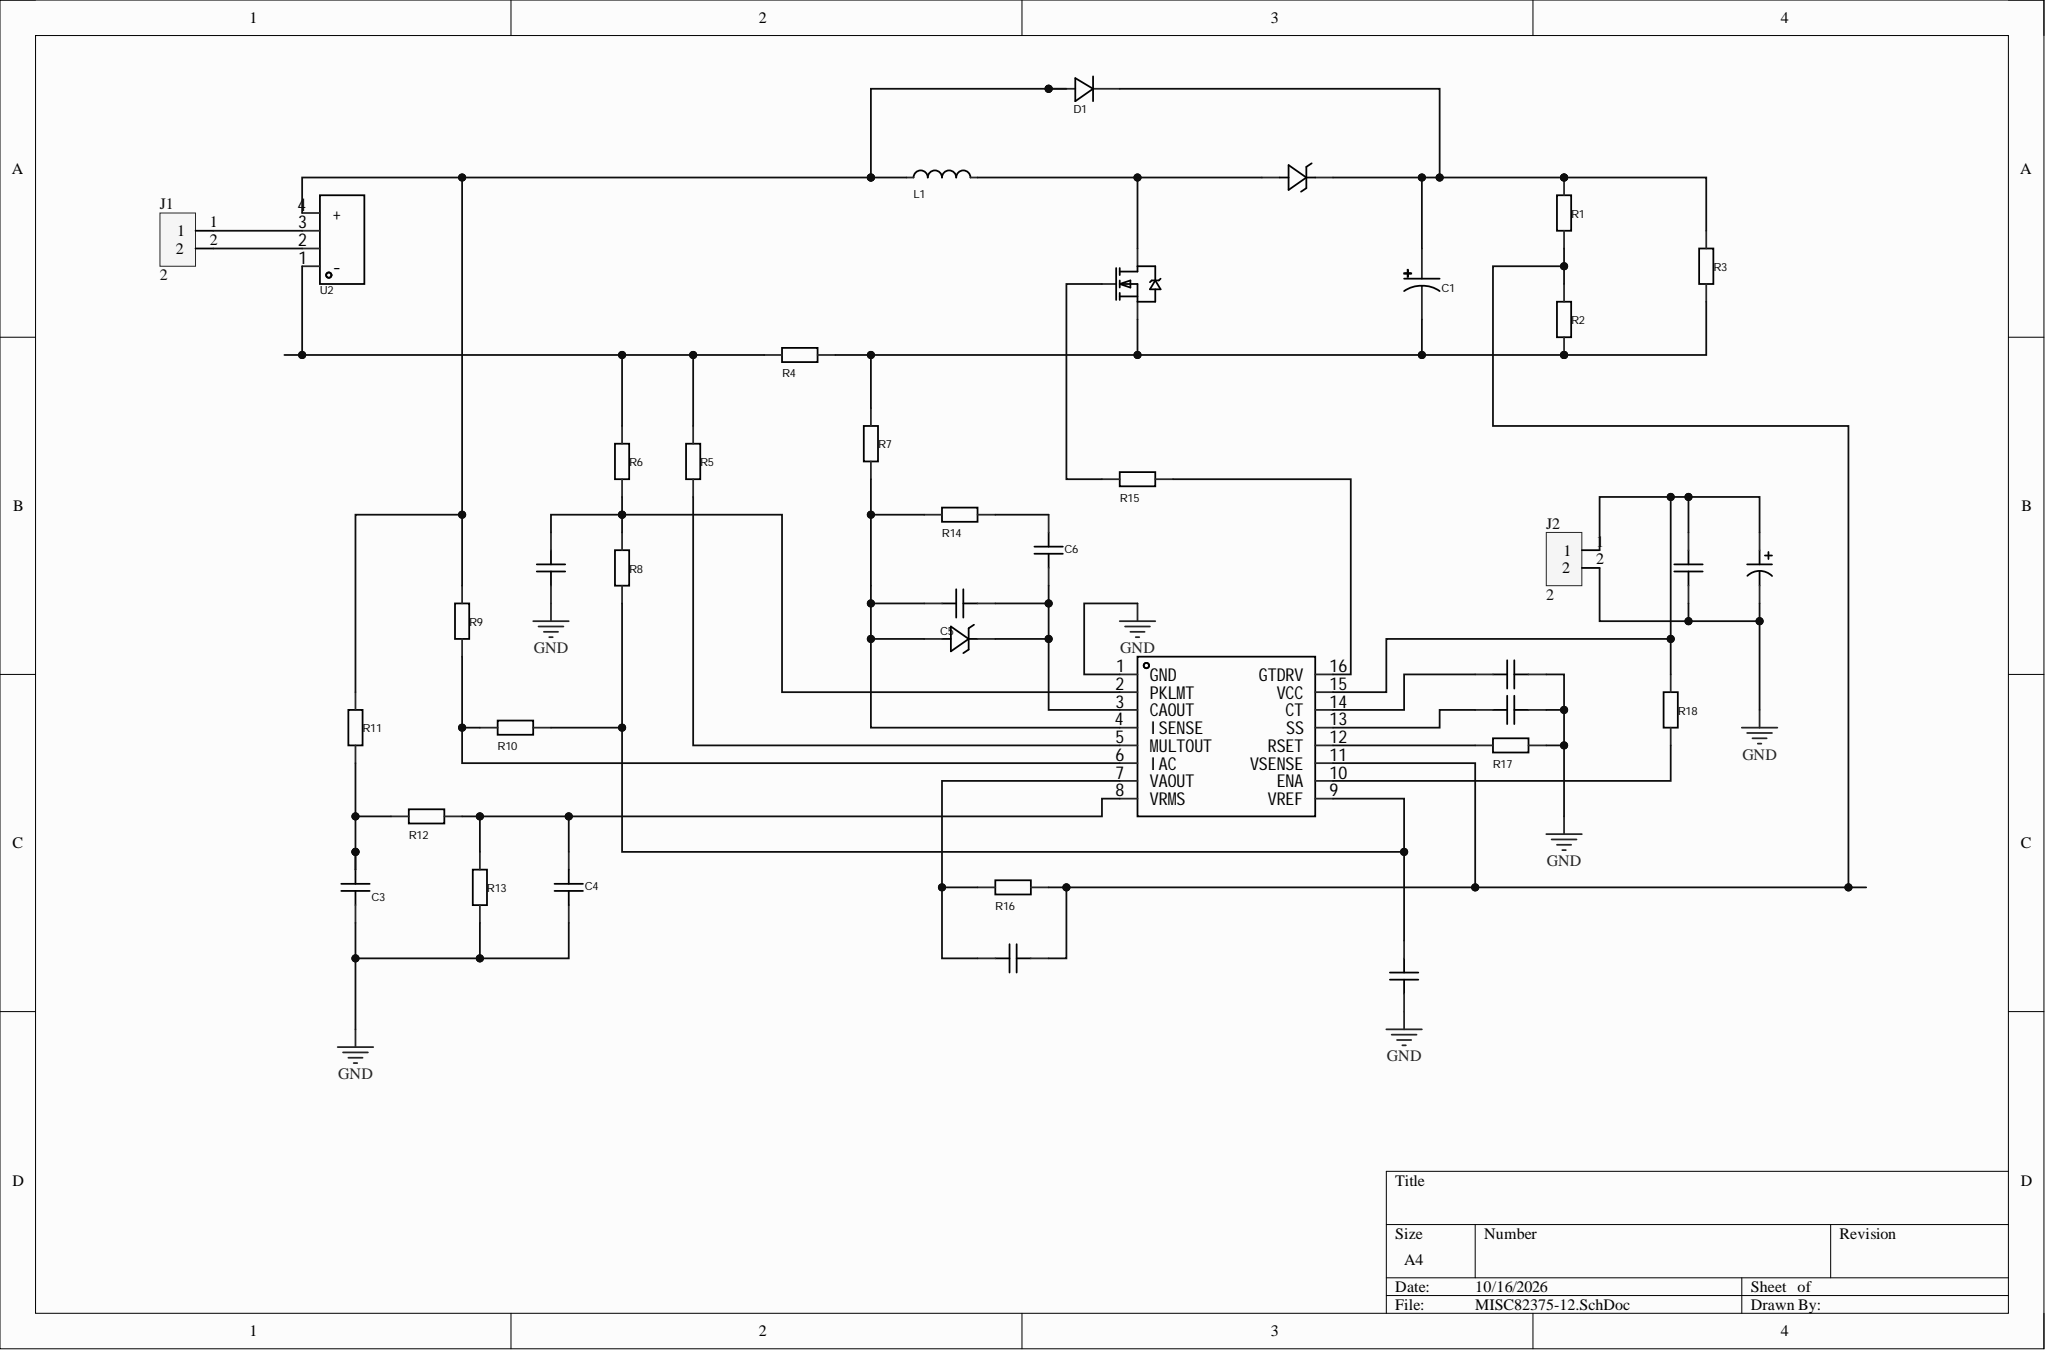Circuit board | Altium Designer | 39 parts | 26 nets
Bill of materials:
Comment,Description,Designator,Footprint,LibRef,Quantity
"LKME1402A101MF","","C1","CAP-TH_BD10.0-P5.00-D1.0-FD","LKME1402A101MF","1"
"KJKF222M2FF7035A075E","","C2","CAP-TH_L6.5-W3.5-P7.50-D1.0","KJKF222M2FF7035A075E","1"
"KY1102M400VAC70Y10093","","C3, C7, C11","CAP-TH_L7.5-W4.5-P10.00-D0.6","KY1102M400VAC70Y10093","3"
"CBB21-400V/255JP20","","C4","CAP-TH_L22.0-W12.5-P20.00-D0.7-FD","CBB21-400V/255JP20","1"
"178MU0002","","C5, C6, C8, C9, C10","CAP-TH_L5.8-W3.6-P5.0-D0.6","178MU0002","5"
"RVE100UF35V67RV0072","","","CAP-SMD_BD6.3-L6.6-W6.6-LS7.6-FD-1","RVE100UF35V67RV0072","1"
"1N5406_C5338388","","D1","DO-27_BD5.2-L8.9-P12.90-D1.5-RD","1N5406_C5338388","1"
"GC3D10060A","","D2","TO-220-2_L10.2-W4.5-P5.08-L-A","GC3D10060A","1"
"BZT52C8V2_C19077406","","D3","SOD-123_L2.7-W1.6-LS3.7-RD","BZT52C8V2_C19077406","1"
"2","","J1, J2","DIP2 - duplicate","AC_in","2"
"XR8*10-101K-L","","L1","IND-TH_BD10.0-P5.00-D0.6","XR8*10-101K-L","1"
"IRF530NPBF","","Q1","TO-220-3_L10.0-W4.5-P2.54-L","IRF530NPBF","1"
"MF1/4W-100K±1%-OT26","","R1, R2, R3, R4, R5, R6, R7, R8, R9, R10, R11, R12, R13, R14, R15, R16, R17, R18","RES-TH_BD2.7-L6.2-P10.20-D0.4","MF1/4W-100K±1%-OT26","18"
"UC3854N","","U1","PDIP-16_L19.3-W6.4-P2.54-LS7.94-BL","UC3854N","1"
"GBU8K","","U2","GBU_4P-L22.0-W3.5-P5.08-GBU4K","GBU8K","1"
Netlist (Protel format):
[
C1
CAP-TH_BD10.0-P5.00-D1.0-FD
LKME1402A101MF



]
[
C2
CAP-TH_L6.5-W3.5-P7.50-D1.0
KJKF222M2FF7035A075E



]
[
C3
CAP-TH_L7.5-W4.5-P10.00-D0.6
KY1102M400VAC70Y10093



]
[
C4
CAP-TH_L22.0-W12.5-P20.00-D0.7-FD
CBB21-400V/255JP20



]
[
C5
CAP-TH_L5.8-W3.6-P5.0-D0.6
178MU0002



]
[
C6
CAP-TH_L5.8-W3.6-P5.0-D0.6
178MU0002



]
[
C7
CAP-TH_L7.5-W4.5-P10.00-D0.6
KY1102M400VAC70Y10093



]
[
C8
CAP-TH_L5.8-W3.6-P5.0-D0.6
178MU0002



]
[
C9
CAP-TH_L5.8-W3.6-P5.0-D0.6
178MU0002



]
[
C10
CAP-TH_L5.8-W3.6-P5.0-D0.6
178MU0002



]
[
C11
CAP-TH_L7.5-W4.5-P10.00-D0.6
KY1102M400VAC70Y10093



]
[
C??
CAP-SMD_BD6.3-L6.6-W6.6-LS7.6-FD-1
RVE100UF35V67RV0072



]
[
D1
DO-27_BD5.2-L8.9-P12.90-D1.5-RD
1N5406_C5338388



]
[
D2
TO-220-2_L10.2-W4.5-P5.08-L-A
GC3D10060A



]
[
D3
SOD-123_L2.7-W1.6-LS3.7-RD
BZT52C8V2_C19077406



]
[
J1
DIP2 - duplicate
2



]
[
J2
DIP2 - duplicate
2



]
[
L1
IND-TH_BD10.0-P5.00-D0.6
XR8*10-101K-L



]
[
Q1
TO-220-3_L10.0-W4.5-P2.54-L
IRF530NPBF



]
[
R1
RES-TH_BD2.7-L6.2-P10.20-D0.4
MF1/4W-100K±1%-OT26



]
[
R2
RES-TH_BD2.7-L6.2-P10.20-D0.4
MF1/4W-100K±1%-OT26



]
[
R3
RES-TH_BD2.7-L6.2-P10.20-D0.4
MF1/4W-100K±1%-OT26



]
[
R4
RES-TH_BD2.7-L6.2-P10.20-D0.4
MF1/4W-100K±1%-OT26



]
[
R5
RES-TH_BD2.7-L6.2-P10.20-D0.4
MF1/4W-100K±1%-OT26



]
[
R6
RES-TH_BD2.7-L6.2-P10.20-D0.4
MF1/4W-100K±1%-OT26



]
[
R7
RES-TH_BD2.7-L6.2-P10.20-D0.4
MF1/4W-100K±1%-OT26



]
[
R8
RES-TH_BD2.7-L6.2-P10.20-D0.4
MF1/4W-100K±1%-OT26



]
[
R9
RES-TH_BD2.7-L6.2-P10.20-D0.4
MF1/4W-100K±1%-OT26



]
[
R10
RES-TH_BD2.7-L6.2-P10.20-D0.4
MF1/4W-100K±1%-OT26



]
[
R11
RES-TH_BD2.7-L6.2-P10.20-D0.4
MF1/4W-100K±1%-OT26



]
[
R12
RES-TH_BD2.7-L6.2-P10.20-D0.4
MF1/4W-100K±1%-OT26



]
[
R13
RES-TH_BD2.7-L6.2-P10.20-D0.4
MF1/4W-100K±1%-OT26



]
[
R14
RES-TH_BD2.7-L6.2-P10.20-D0.4
MF1/4W-100K±1%-OT26



]
[
R15
RES-TH_BD2.7-L6.2-P10.20-D0.4
MF1/4W-100K±1%-OT26



]
[
R16
RES-TH_BD2.7-L6.2-P10.20-D0.4
MF1/4W-100K±1%-OT26



]
[
R17
RES-TH_BD2.7-L6.2-P10.20-D0.4
MF1/4W-100K±1%-OT26



]
[
R18
RES-TH_BD2.7-L6.2-P10.20-D0.4
MF1/4W-100K±1%-OT26



]
[
U1
PDIP-16_L19.3-W6.4-P2.54-LS7.94-BL
UC3854N



]
[
U2
GBU_4P-L22.0-W3.5-P5.08-GBU4K
GBU8K



]
(
NetR18_1
R18-1
U1-10
)
(
NetR17_1
R17-1
U1-12
)
(
NetR15_2
R15-2
U1-16
)
(
NetR9_1
R9-1
R10-1
U1-6
)
(
NetR5_1
R5-1
U1-5
)
(
NetR4_1
R4-1
R5-2
R6-2
U2-1
)
(
NetQ1_1
Q1-1
R15-1
)
(
NetJ1_2
J1-2
U2-2
)
(
NetJ1_1
J1-1
U2-3
)
(
NetD2_3
D2-3
L1-2
Q1-2
)
(
NetD1_2
D1-2
L1-1
R9-2
R11-2
U2-4
)
(
NetC11_2
C11-2
C??-1
J2-1
R18-2
U1-15
)
(
NetC10_1
C10-1
U1-14
)
(
NetC9_1
C9-1
U1-13
)
(
NetC8_2
C8-2
R8-1
R10-2
U1-9
)
(
NetC7_2
C7-2
R1-1
R2-2
R16-2
U1-11
)
(
NetC7_1
C7-1
R16-1
U1-7
)
(
NetC6_2
C6-2
R14-2
)
(
NetC5_2
C5-2
C6-1
D3-1
U1-3
)
(
NetC5_1
C5-1
D3-2
R7-1
R14-1
U1-4
)
(
NetC4_2
C4-2
R12-2
R13-2
U1-8
)
(
NetC3_2
C3-2
R11-1
R12-1
)
(
NetC2_2
C2-2
R6-1
R8-2
U1-2
)
(
NetC1_2
C1-2
Q1-3
R2-1
R3-1
R4-2
R7-2
)
(
NetC1_1
C1-1
D1-1
D2-1
R1-2
R3-2
)
(
GND
C2-1
C3-1
C4-1
C8-1
C9-2
C10-2
C11-1
C??-2
J2-2
R13-1
R17-2
U1-1
)